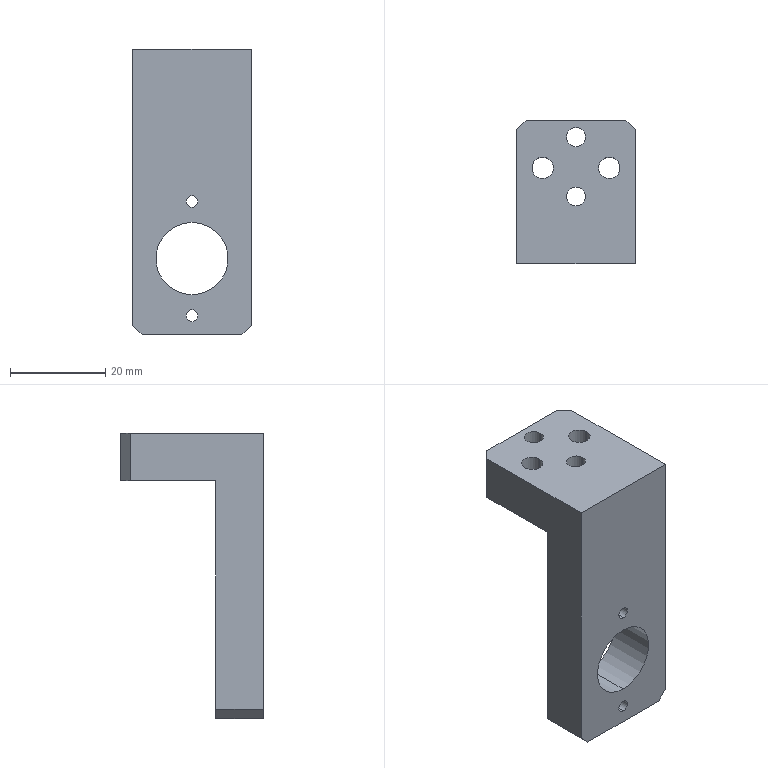Part | SolidWorks | features HoleWzd 3, ICE 2, Chamfer 1, Extrusion 1 | 1 solid | 32 faces | box 25 x 30 x 60 mm | volume 17122 mm3 | cylinder 18 | plane 14 | commonest cylinder face diameters 2.5 x4 4 x4 4.5 x4 8 x4 15.2 x2
STEP:
#1=CARTESIAN_POINT('',(0.,10.,-27.25));
#2=VERTEX_POINT('',#1);
#3=CARTESIAN_POINT('',(0.,10.,-24.75));
#4=VERTEX_POINT('',#3);
#5=CARTESIAN_POINT('',(0.,10.,-26.));
#6=DIRECTION('',(0.,1.,0.));
#7=DIRECTION('',(0.,0.,1.));
#8=AXIS2_PLACEMENT_3D('',#5,#6,#7);
#9=CIRCLE('',#8,1.25);
#10=EDGE_CURVE('',#2,#4,#9,.T.);
#11=ORIENTED_EDGE('',*,*,#10,.T.);
#12=CARTESIAN_POINT('',(0.,0.,-24.75));
#13=VERTEX_POINT('',#12);
#14=CARTESIAN_POINT('',(0.,0.,-24.75));
#15=DIRECTION('',(0.,-1.,0.));
#16=VECTOR('',#15,1000.);
#17=LINE('',#14,#16);
#18=EDGE_CURVE('',#4,#13,#17,.T.);
#19=ORIENTED_EDGE('',*,*,#18,.T.);
#20=CARTESIAN_POINT('',(0.,0.,-27.25));
#21=VERTEX_POINT('',#20);
#22=CARTESIAN_POINT('',(0.,0.,-26.));
#23=DIRECTION('',(0.,-1.,0.));
#24=DIRECTION('',(0.,0.,-1.));
#25=AXIS2_PLACEMENT_3D('',#22,#23,#24);
#26=CIRCLE('',#25,1.25);
#27=EDGE_CURVE('',#13,#21,#26,.T.);
#28=ORIENTED_EDGE('',*,*,#27,.T.);
#29=CARTESIAN_POINT('',(0.,0.,-27.25));
#30=DIRECTION('',(0.,-1.,0.));
#31=VECTOR('',#30,1000.);
#32=LINE('',#29,#31);
#33=EDGE_CURVE('',#2,#21,#32,.T.);
#34=ORIENTED_EDGE('',*,*,#33,.F.);
#35=EDGE_LOOP('',(#11,#19,#28,#34));
#36=FACE_OUTER_BOUND('',#35,.T.);
#37=CARTESIAN_POINT('',(0.,0.,-26.));
#38=DIRECTION('',(0.,-1.,0.));
#39=DIRECTION('',(0.,0.,-1.));
#40=AXIS2_PLACEMENT_3D('',#37,#38,#39);
#41=CYLINDRICAL_SURFACE('',#40,1.25);
#42=ADVANCED_FACE('',(#36),#41,.F.);
#43=CARTESIAN_POINT('',(0.,10.,-3.25));
#44=VERTEX_POINT('',#43);
#45=CARTESIAN_POINT('',(0.,10.,-0.75));
#46=VERTEX_POINT('',#45);
#47=CARTESIAN_POINT('',(0.,10.,-2.));
#48=DIRECTION('',(0.,1.,0.));
#49=DIRECTION('',(0.,0.,1.));
#50=AXIS2_PLACEMENT_3D('',#47,#48,#49);
#51=CIRCLE('',#50,1.25);
#52=EDGE_CURVE('',#44,#46,#51,.T.);
#53=ORIENTED_EDGE('',*,*,#52,.T.);
#54=CARTESIAN_POINT('',(0.,0.,-0.75));
#55=VERTEX_POINT('',#54);
#56=CARTESIAN_POINT('',(0.,0.,-0.75));
#57=DIRECTION('',(0.,-1.,0.));
#58=VECTOR('',#57,1000.);
#59=LINE('',#56,#58);
#60=EDGE_CURVE('',#46,#55,#59,.T.);
#61=ORIENTED_EDGE('',*,*,#60,.T.);
#62=CARTESIAN_POINT('',(0.,0.,-3.25));
#63=VERTEX_POINT('',#62);
#64=CARTESIAN_POINT('',(0.,0.,-2.));
#65=DIRECTION('',(0.,-1.,0.));
#66=DIRECTION('',(0.,0.,-1.));
#67=AXIS2_PLACEMENT_3D('',#64,#65,#66);
#68=CIRCLE('',#67,1.25);
#69=EDGE_CURVE('',#55,#63,#68,.T.);
#70=ORIENTED_EDGE('',*,*,#69,.T.);
#71=CARTESIAN_POINT('',(0.,0.,-3.25));
#72=DIRECTION('',(0.,-1.,0.));
#73=VECTOR('',#72,1000.);
#74=LINE('',#71,#73);
#75=EDGE_CURVE('',#44,#63,#74,.T.);
#76=ORIENTED_EDGE('',*,*,#75,.F.);
#77=EDGE_LOOP('',(#53,#61,#70,#76));
#78=FACE_OUTER_BOUND('',#77,.T.);
#79=CARTESIAN_POINT('',(0.,0.,-2.));
#80=DIRECTION('',(0.,-1.,0.));
#81=DIRECTION('',(0.,0.,-1.));
#82=AXIS2_PLACEMENT_3D('',#79,#80,#81);
#83=CYLINDRICAL_SURFACE('',#82,1.25);
#84=ADVANCED_FACE('',(#78),#83,.F.);
#85=CARTESIAN_POINT('',(2.,26.5,30.));
#86=VERTEX_POINT('',#85);
#87=CARTESIAN_POINT('',(-2.,26.5,30.));
#88=VERTEX_POINT('',#87);
#89=CARTESIAN_POINT('',(0.,26.5,30.));
#90=DIRECTION('',(0.,0.,-1.));
#91=DIRECTION('',(-1.,0.,0.));
#92=AXIS2_PLACEMENT_3D('',#89,#90,#91);
#93=CIRCLE('',#92,2.);
#94=EDGE_CURVE('',#86,#88,#93,.T.);
#95=ORIENTED_EDGE('',*,*,#94,.F.);
#96=CARTESIAN_POINT('',(2.,26.5,20.));
#97=VERTEX_POINT('',#96);
#98=CARTESIAN_POINT('',(2.,26.5,20.));
#99=DIRECTION('',(0.,0.,-1.));
#100=VECTOR('',#99,1000.);
#101=LINE('',#98,#100);
#102=EDGE_CURVE('',#86,#97,#101,.T.);
#103=ORIENTED_EDGE('',*,*,#102,.T.);
#104=CARTESIAN_POINT('',(-2.,26.5,20.));
#105=VERTEX_POINT('',#104);
#106=CARTESIAN_POINT('',(0.,26.5,20.));
#107=DIRECTION('',(0.,0.,-1.));
#108=DIRECTION('',(-1.,0.,0.));
#109=AXIS2_PLACEMENT_3D('',#106,#107,#108);
#110=CIRCLE('',#109,2.);
#111=EDGE_CURVE('',#97,#105,#110,.T.);
#112=ORIENTED_EDGE('',*,*,#111,.T.);
#113=CARTESIAN_POINT('',(-2.,26.5,20.));
#114=DIRECTION('',(0.,0.,-1.));
#115=VECTOR('',#114,1000.);
#116=LINE('',#113,#115);
#117=EDGE_CURVE('',#88,#105,#116,.T.);
#118=ORIENTED_EDGE('',*,*,#117,.F.);
#119=EDGE_LOOP('',(#95,#103,#112,#118));
#120=FACE_OUTER_BOUND('',#119,.T.);
#121=CARTESIAN_POINT('',(0.,26.5,20.));
#122=DIRECTION('',(0.,0.,-1.));
#123=DIRECTION('',(-1.,0.,0.));
#124=AXIS2_PLACEMENT_3D('',#121,#122,#123);
#125=CYLINDRICAL_SURFACE('',#124,2.);
#126=ADVANCED_FACE('',(#120),#125,.F.);
#127=CARTESIAN_POINT('',(2.,14.,30.));
#128=VERTEX_POINT('',#127);
#129=CARTESIAN_POINT('',(-2.,14.,30.));
#130=VERTEX_POINT('',#129);
#131=CARTESIAN_POINT('',(0.,14.,30.));
#132=DIRECTION('',(0.,0.,-1.));
#133=DIRECTION('',(-1.,0.,0.));
#134=AXIS2_PLACEMENT_3D('',#131,#132,#133);
#135=CIRCLE('',#134,2.);
#136=EDGE_CURVE('',#128,#130,#135,.T.);
#137=ORIENTED_EDGE('',*,*,#136,.F.);
#138=CARTESIAN_POINT('',(2.,14.,20.));
#139=VERTEX_POINT('',#138);
#140=CARTESIAN_POINT('',(2.,14.,20.));
#141=DIRECTION('',(0.,0.,-1.));
#142=VECTOR('',#141,1000.);
#143=LINE('',#140,#142);
#144=EDGE_CURVE('',#128,#139,#143,.T.);
#145=ORIENTED_EDGE('',*,*,#144,.T.);
#146=CARTESIAN_POINT('',(-2.,14.,20.));
#147=VERTEX_POINT('',#146);
#148=CARTESIAN_POINT('',(0.,14.,20.));
#149=DIRECTION('',(0.,0.,-1.));
#150=DIRECTION('',(-1.,0.,0.));
#151=AXIS2_PLACEMENT_3D('',#148,#149,#150);
#152=CIRCLE('',#151,2.);
#153=EDGE_CURVE('',#139,#147,#152,.T.);
#154=ORIENTED_EDGE('',*,*,#153,.T.);
#155=CARTESIAN_POINT('',(-2.,14.,20.));
#156=DIRECTION('',(0.,0.,-1.));
#157=VECTOR('',#156,1000.);
#158=LINE('',#155,#157);
#159=EDGE_CURVE('',#130,#147,#158,.T.);
#160=ORIENTED_EDGE('',*,*,#159,.F.);
#161=EDGE_LOOP('',(#137,#145,#154,#160));
#162=FACE_OUTER_BOUND('',#161,.T.);
#163=CARTESIAN_POINT('',(0.,14.,20.));
#164=DIRECTION('',(0.,0.,-1.));
#165=DIRECTION('',(-1.,0.,0.));
#166=AXIS2_PLACEMENT_3D('',#163,#164,#165);
#167=CYLINDRICAL_SURFACE('',#166,2.);
#168=ADVANCED_FACE('',(#162),#167,.F.);
#169=CARTESIAN_POINT('',(-3.,20.,24.6));
#170=VERTEX_POINT('',#169);
#171=CARTESIAN_POINT('',(-11.,20.,24.6));
#172=VERTEX_POINT('',#171);
#173=CARTESIAN_POINT('',(-7.,20.,24.6));
#174=DIRECTION('',(0.,0.,-1.));
#175=DIRECTION('',(-1.,0.,0.));
#176=AXIS2_PLACEMENT_3D('',#173,#174,#175);
#177=CIRCLE('',#176,4.);
#178=EDGE_CURVE('',#170,#172,#177,.T.);
#179=ORIENTED_EDGE('',*,*,#178,.F.);
#180=CARTESIAN_POINT('',(-3.,20.,20.));
#181=VERTEX_POINT('',#180);
#182=CARTESIAN_POINT('',(-3.,20.,20.));
#183=DIRECTION('',(0.,0.,-1.));
#184=VECTOR('',#183,1000.);
#185=LINE('',#182,#184);
#186=EDGE_CURVE('',#170,#181,#185,.T.);
#187=ORIENTED_EDGE('',*,*,#186,.T.);
#188=CARTESIAN_POINT('',(-11.,20.,20.));
#189=VERTEX_POINT('',#188);
#190=CARTESIAN_POINT('',(-7.,20.,20.));
#191=DIRECTION('',(0.,0.,-1.));
#192=DIRECTION('',(-1.,0.,0.));
#193=AXIS2_PLACEMENT_3D('',#190,#191,#192);
#194=CIRCLE('',#193,4.);
#195=EDGE_CURVE('',#181,#189,#194,.T.);
#196=ORIENTED_EDGE('',*,*,#195,.T.);
#197=CARTESIAN_POINT('',(-11.,20.,20.));
#198=DIRECTION('',(0.,0.,-1.));
#199=VECTOR('',#198,1000.);
#200=LINE('',#197,#199);
#201=EDGE_CURVE('',#172,#189,#200,.T.);
#202=ORIENTED_EDGE('',*,*,#201,.F.);
#203=EDGE_LOOP('',(#179,#187,#196,#202));
#204=FACE_OUTER_BOUND('',#203,.T.);
#205=CARTESIAN_POINT('',(-7.,20.,20.));
#206=DIRECTION('',(0.,0.,-1.));
#207=DIRECTION('',(-1.,0.,0.));
#208=AXIS2_PLACEMENT_3D('',#205,#206,#207);
#209=CYLINDRICAL_SURFACE('',#208,4.);
#210=ADVANCED_FACE('',(#204),#209,.F.);
#211=CARTESIAN_POINT('',(-4.75,20.,30.));
#212=VERTEX_POINT('',#211);
#213=CARTESIAN_POINT('',(-9.25,20.,30.));
#214=VERTEX_POINT('',#213);
#215=CARTESIAN_POINT('',(-7.,20.,30.));
#216=DIRECTION('',(0.,0.,-1.));
#217=DIRECTION('',(-1.,0.,0.));
#218=AXIS2_PLACEMENT_3D('',#215,#216,#217);
#219=CIRCLE('',#218,2.25);
#220=EDGE_CURVE('',#212,#214,#219,.T.);
#221=ORIENTED_EDGE('',*,*,#220,.F.);
#222=CARTESIAN_POINT('',(-4.75,20.,24.6));
#223=VERTEX_POINT('',#222);
#224=CARTESIAN_POINT('',(-4.75,20.,20.));
#225=DIRECTION('',(0.,0.,-1.));
#226=VECTOR('',#225,1000.);
#227=LINE('',#224,#226);
#228=EDGE_CURVE('',#212,#223,#227,.T.);
#229=ORIENTED_EDGE('',*,*,#228,.T.);
#230=CARTESIAN_POINT('',(-9.25,20.,24.6));
#231=VERTEX_POINT('',#230);
#232=CARTESIAN_POINT('',(-7.,20.,24.6));
#233=DIRECTION('',(0.,0.,-1.));
#234=DIRECTION('',(-1.,0.,0.));
#235=AXIS2_PLACEMENT_3D('',#232,#233,#234);
#236=CIRCLE('',#235,2.25);
#237=EDGE_CURVE('',#223,#231,#236,.T.);
#238=ORIENTED_EDGE('',*,*,#237,.T.);
#239=CARTESIAN_POINT('',(-9.25,20.,20.));
#240=DIRECTION('',(0.,0.,-1.));
#241=VECTOR('',#240,1000.);
#242=LINE('',#239,#241);
#243=EDGE_CURVE('',#214,#231,#242,.T.);
#244=ORIENTED_EDGE('',*,*,#243,.F.);
#245=EDGE_LOOP('',(#221,#229,#238,#244));
#246=FACE_OUTER_BOUND('',#245,.T.);
#247=CARTESIAN_POINT('',(-7.,20.,20.));
#248=DIRECTION('',(0.,0.,-1.));
#249=DIRECTION('',(-1.,0.,0.));
#250=AXIS2_PLACEMENT_3D('',#247,#248,#249);
#251=CYLINDRICAL_SURFACE('',#250,2.25);
#252=ADVANCED_FACE('',(#246),#251,.F.);
#253=CARTESIAN_POINT('',(11.,20.,24.6));
#254=VERTEX_POINT('',#253);
#255=CARTESIAN_POINT('',(3.,20.,24.6));
#256=VERTEX_POINT('',#255);
#257=CARTESIAN_POINT('',(7.,20.,24.6));
#258=DIRECTION('',(0.,0.,-1.));
#259=DIRECTION('',(-1.,0.,0.));
#260=AXIS2_PLACEMENT_3D('',#257,#258,#259);
#261=CIRCLE('',#260,4.);
#262=EDGE_CURVE('',#254,#256,#261,.T.);
#263=ORIENTED_EDGE('',*,*,#262,.F.);
#264=CARTESIAN_POINT('',(11.,20.,20.));
#265=VERTEX_POINT('',#264);
#266=CARTESIAN_POINT('',(11.,20.,20.));
#267=DIRECTION('',(0.,0.,-1.));
#268=VECTOR('',#267,1000.);
#269=LINE('',#266,#268);
#270=EDGE_CURVE('',#254,#265,#269,.T.);
#271=ORIENTED_EDGE('',*,*,#270,.T.);
#272=CARTESIAN_POINT('',(3.,20.,20.));
#273=VERTEX_POINT('',#272);
#274=CARTESIAN_POINT('',(7.,20.,20.));
#275=DIRECTION('',(0.,0.,-1.));
#276=DIRECTION('',(-1.,0.,0.));
#277=AXIS2_PLACEMENT_3D('',#274,#275,#276);
#278=CIRCLE('',#277,4.);
#279=EDGE_CURVE('',#265,#273,#278,.T.);
#280=ORIENTED_EDGE('',*,*,#279,.T.);
#281=CARTESIAN_POINT('',(3.,20.,20.));
#282=DIRECTION('',(0.,0.,-1.));
#283=VECTOR('',#282,1000.);
#284=LINE('',#281,#283);
#285=EDGE_CURVE('',#256,#273,#284,.T.);
#286=ORIENTED_EDGE('',*,*,#285,.F.);
#287=EDGE_LOOP('',(#263,#271,#280,#286));
#288=FACE_OUTER_BOUND('',#287,.T.);
#289=CARTESIAN_POINT('',(7.,20.,20.));
#290=DIRECTION('',(0.,0.,-1.));
#291=DIRECTION('',(-1.,0.,0.));
#292=AXIS2_PLACEMENT_3D('',#289,#290,#291);
#293=CYLINDRICAL_SURFACE('',#292,4.);
#294=ADVANCED_FACE('',(#288),#293,.F.);
#295=CARTESIAN_POINT('',(9.25,20.,30.));
#296=VERTEX_POINT('',#295);
#297=CARTESIAN_POINT('',(4.75,20.,30.));
#298=VERTEX_POINT('',#297);
#299=CARTESIAN_POINT('',(7.,20.,30.));
#300=DIRECTION('',(0.,0.,-1.));
#301=DIRECTION('',(-1.,0.,0.));
#302=AXIS2_PLACEMENT_3D('',#299,#300,#301);
#303=CIRCLE('',#302,2.25);
#304=EDGE_CURVE('',#296,#298,#303,.T.);
#305=ORIENTED_EDGE('',*,*,#304,.F.);
#306=CARTESIAN_POINT('',(9.25,20.,24.6));
#307=VERTEX_POINT('',#306);
#308=CARTESIAN_POINT('',(9.25,20.,20.));
#309=DIRECTION('',(0.,0.,-1.));
#310=VECTOR('',#309,1000.);
#311=LINE('',#308,#310);
#312=EDGE_CURVE('',#296,#307,#311,.T.);
#313=ORIENTED_EDGE('',*,*,#312,.T.);
#314=CARTESIAN_POINT('',(4.75,20.,24.6));
#315=VERTEX_POINT('',#314);
#316=CARTESIAN_POINT('',(7.,20.,24.6));
#317=DIRECTION('',(0.,0.,-1.));
#318=DIRECTION('',(-1.,0.,0.));
#319=AXIS2_PLACEMENT_3D('',#316,#317,#318);
#320=CIRCLE('',#319,2.25);
#321=EDGE_CURVE('',#307,#315,#320,.T.);
#322=ORIENTED_EDGE('',*,*,#321,.T.);
#323=CARTESIAN_POINT('',(4.75,20.,20.));
#324=DIRECTION('',(0.,0.,-1.));
#325=VECTOR('',#324,1000.);
#326=LINE('',#323,#325);
#327=EDGE_CURVE('',#298,#315,#326,.T.);
#328=ORIENTED_EDGE('',*,*,#327,.F.);
#329=EDGE_LOOP('',(#305,#313,#322,#328));
#330=FACE_OUTER_BOUND('',#329,.T.);
#331=CARTESIAN_POINT('',(7.,20.,20.));
#332=DIRECTION('',(0.,0.,-1.));
#333=DIRECTION('',(-1.,0.,0.));
#334=AXIS2_PLACEMENT_3D('',#331,#332,#333);
#335=CYLINDRICAL_SURFACE('',#334,2.25);
#336=ADVANCED_FACE('',(#330),#335,.F.);
#337=CARTESIAN_POINT('',(0.,10.,-21.6));
#338=VERTEX_POINT('',#337);
#339=CARTESIAN_POINT('',(0.,10.,-6.4));
#340=VERTEX_POINT('',#339);
#341=CARTESIAN_POINT('',(0.,10.,-14.));
#342=DIRECTION('',(0.,1.,0.));
#343=DIRECTION('',(0.,0.,1.));
#344=AXIS2_PLACEMENT_3D('',#341,#342,#343);
#345=CIRCLE('',#344,7.6);
#346=EDGE_CURVE('',#338,#340,#345,.T.);
#347=ORIENTED_EDGE('',*,*,#346,.T.);
#348=CARTESIAN_POINT('',(0.,0.,-6.4));
#349=VERTEX_POINT('',#348);
#350=CARTESIAN_POINT('',(0.,20.,-6.4));
#351=DIRECTION('',(0.,-1.,0.));
#352=VECTOR('',#351,1000.);
#353=LINE('',#350,#352);
#354=EDGE_CURVE('',#340,#349,#353,.T.);
#355=ORIENTED_EDGE('',*,*,#354,.T.);
#356=CARTESIAN_POINT('',(0.,0.,-21.6));
#357=VERTEX_POINT('',#356);
#358=CARTESIAN_POINT('',(0.,0.,-14.));
#359=DIRECTION('',(0.,-1.,0.));
#360=DIRECTION('',(0.,0.,-1.));
#361=AXIS2_PLACEMENT_3D('',#358,#359,#360);
#362=CIRCLE('',#361,7.6);
#363=EDGE_CURVE('',#349,#357,#362,.T.);
#364=ORIENTED_EDGE('',*,*,#363,.T.);
#365=CARTESIAN_POINT('',(0.,20.,-21.6));
#366=DIRECTION('',(0.,-1.,0.));
#367=VECTOR('',#366,1000.);
#368=LINE('',#365,#367);
#369=EDGE_CURVE('',#338,#357,#368,.T.);
#370=ORIENTED_EDGE('',*,*,#369,.F.);
#371=EDGE_LOOP('',(#347,#355,#364,#370));
#372=FACE_OUTER_BOUND('',#371,.T.);
#373=CARTESIAN_POINT('',(0.,20.,-14.));
#374=DIRECTION('',(0.,-1.,0.));
#375=DIRECTION('',(0.,0.,-1.));
#376=AXIS2_PLACEMENT_3D('',#373,#374,#375);
#377=CYLINDRICAL_SURFACE('',#376,7.6);
#378=ADVANCED_FACE('',(#372),#377,.F.);
#379=CARTESIAN_POINT('',(12.5,28.,20.));
#380=VERTEX_POINT('',#379);
#381=CARTESIAN_POINT('',(12.5,10.,20.));
#382=VERTEX_POINT('',#381);
#383=CARTESIAN_POINT('',(12.5,30.,20.));
#384=DIRECTION('',(0.,-1.,0.));
#385=VECTOR('',#384,1000.);
#386=LINE('',#383,#385);
#387=EDGE_CURVE('',#380,#382,#386,.T.);
#388=ORIENTED_EDGE('',*,*,#387,.F.);
#389=CARTESIAN_POINT('',(12.5,28.,30.));
#390=VERTEX_POINT('',#389);
#391=CARTESIAN_POINT('',(12.5,28.,-30.));
#392=DIRECTION('',(0.,0.,1.));
#393=VECTOR('',#392,1000.);
#394=LINE('',#391,#393);
#395=EDGE_CURVE('',#380,#390,#394,.T.);
#396=ORIENTED_EDGE('',*,*,#395,.T.);
#397=CARTESIAN_POINT('',(12.5,0.,30.));
#398=VERTEX_POINT('',#397);
#399=CARTESIAN_POINT('',(12.5,10.,30.));
#400=DIRECTION('',(0.,-1.,0.));
#401=VECTOR('',#400,1000.);
#402=LINE('',#399,#401);
#403=EDGE_CURVE('',#390,#398,#402,.T.);
#404=ORIENTED_EDGE('',*,*,#403,.T.);
#405=CARTESIAN_POINT('',(12.5,0.,-28.));
#406=VERTEX_POINT('',#405);
#407=CARTESIAN_POINT('',(12.5,0.,-30.));
#408=DIRECTION('',(0.,0.,-1.));
#409=VECTOR('',#408,1000.);
#410=LINE('',#407,#409);
#411=EDGE_CURVE('',#398,#406,#410,.T.);
#412=ORIENTED_EDGE('',*,*,#411,.T.);
#413=CARTESIAN_POINT('',(12.5,10.,-28.));
#414=VERTEX_POINT('',#413);
#415=CARTESIAN_POINT('',(12.5,10.,-28.));
#416=DIRECTION('',(0.,1.,0.));
#417=VECTOR('',#416,1000.);
#418=LINE('',#415,#417);
#419=EDGE_CURVE('',#406,#414,#418,.T.);
#420=ORIENTED_EDGE('',*,*,#419,.T.);
#421=CARTESIAN_POINT('',(12.5,10.,-30.));
#422=DIRECTION('',(0.,0.,-1.));
#423=VECTOR('',#422,1000.);
#424=LINE('',#421,#423);
#425=EDGE_CURVE('',#382,#414,#424,.T.);
#426=ORIENTED_EDGE('',*,*,#425,.F.);
#427=EDGE_LOOP('',(#388,#396,#404,#412,#420,#426));
#428=FACE_OUTER_BOUND('',#427,.T.);
#429=CARTESIAN_POINT('',(12.5,10.,-30.));
#430=DIRECTION('',(-1.,0.,0.));
#431=DIRECTION('',(0.,0.,1.));
#432=AXIS2_PLACEMENT_3D('',#429,#430,#431);
#433=PLANE('',#432);
#434=ADVANCED_FACE('',(#428),#433,.F.);
#435=CARTESIAN_POINT('',(10.5,0.,-30.));
#436=VERTEX_POINT('',#435);
#437=CARTESIAN_POINT('',(-10.5,0.,-30.));
#438=VERTEX_POINT('',#437);
#439=CARTESIAN_POINT('',(-12.5,0.,-30.));
#440=DIRECTION('',(-1.,0.,0.));
#441=VECTOR('',#440,1000.);
#442=LINE('',#439,#441);
#443=EDGE_CURVE('',#436,#438,#442,.T.);
#444=ORIENTED_EDGE('',*,*,#443,.T.);
#445=CARTESIAN_POINT('',(-10.5,10.,-30.));
#446=VERTEX_POINT('',#445);
#447=CARTESIAN_POINT('',(-10.5,10.,-30.));
#448=DIRECTION('',(0.,1.,0.));
#449=VECTOR('',#448,1000.);
#450=LINE('',#447,#449);
#451=EDGE_CURVE('',#438,#446,#450,.T.);
#452=ORIENTED_EDGE('',*,*,#451,.T.);
#453=CARTESIAN_POINT('',(10.5,10.,-30.));
#454=VERTEX_POINT('',#453);
#455=CARTESIAN_POINT('',(-12.5,10.,-30.));
#456=DIRECTION('',(-1.,0.,0.));
#457=VECTOR('',#456,1000.);
#458=LINE('',#455,#457);
#459=EDGE_CURVE('',#454,#446,#458,.T.);
#460=ORIENTED_EDGE('',*,*,#459,.F.);
#461=CARTESIAN_POINT('',(10.5,10.,-30.));
#462=DIRECTION('',(0.,-1.,0.));
#463=VECTOR('',#462,1000.);
#464=LINE('',#461,#463);
#465=EDGE_CURVE('',#454,#436,#464,.T.);
#466=ORIENTED_EDGE('',*,*,#465,.T.);
#467=EDGE_LOOP('',(#444,#452,#460,#466));
#468=FACE_OUTER_BOUND('',#467,.T.);
#469=CARTESIAN_POINT('',(-12.5,10.,-30.));
#470=DIRECTION('',(0.,0.,1.));
#471=DIRECTION('',(1.,0.,0.));
#472=AXIS2_PLACEMENT_3D('',#469,#470,#471);
#473=PLANE('',#472);
#474=ADVANCED_FACE('',(#468),#473,.F.);
#475=CARTESIAN_POINT('',(-12.5,28.,30.));
#476=VERTEX_POINT('',#475);
#477=CARTESIAN_POINT('',(-12.5,0.,30.));
#478=VERTEX_POINT('',#477);
#479=CARTESIAN_POINT('',(-12.5,10.,30.));
#480=DIRECTION('',(0.,-1.,0.));
#481=VECTOR('',#480,1000.);
#482=LINE('',#479,#481);
#483=EDGE_CURVE('',#476,#478,#482,.T.);
#484=ORIENTED_EDGE('',*,*,#483,.F.);
#485=CARTESIAN_POINT('',(-12.5,28.,20.));
#486=VERTEX_POINT('',#485);
#487=CARTESIAN_POINT('',(-12.5,28.,-30.));
#488=DIRECTION('',(0.,0.,-1.));
#489=VECTOR('',#488,1000.);
#490=LINE('',#487,#489);
#491=EDGE_CURVE('',#476,#486,#490,.T.);
#492=ORIENTED_EDGE('',*,*,#491,.T.);
#493=CARTESIAN_POINT('',(-12.5,10.,20.));
#494=VERTEX_POINT('',#493);
#495=CARTESIAN_POINT('',(-12.5,30.,20.));
#496=DIRECTION('',(0.,-1.,0.));
#497=VECTOR('',#496,1000.);
#498=LINE('',#495,#497);
#499=EDGE_CURVE('',#486,#494,#498,.T.);
#500=ORIENTED_EDGE('',*,*,#499,.T.);
#501=CARTESIAN_POINT('',(-12.5,10.,-28.));
#502=VERTEX_POINT('',#501);
#503=CARTESIAN_POINT('',(-12.5,10.,-30.));
#504=DIRECTION('',(0.,0.,1.));
#505=VECTOR('',#504,1000.);
#506=LINE('',#503,#505);
#507=EDGE_CURVE('',#502,#494,#506,.T.);
#508=ORIENTED_EDGE('',*,*,#507,.F.);
#509=CARTESIAN_POINT('',(-12.5,0.,-28.));
#510=VERTEX_POINT('',#509);
#511=CARTESIAN_POINT('',(-12.5,10.,-28.));
#512=DIRECTION('',(0.,-1.,0.));
#513=VECTOR('',#512,1000.);
#514=LINE('',#511,#513);
#515=EDGE_CURVE('',#502,#510,#514,.T.);
#516=ORIENTED_EDGE('',*,*,#515,.T.);
#517=CARTESIAN_POINT('',(-12.5,0.,-30.));
#518=DIRECTION('',(0.,0.,1.));
#519=VECTOR('',#518,1000.);
#520=LINE('',#517,#519);
#521=EDGE_CURVE('',#510,#478,#520,.T.);
#522=ORIENTED_EDGE('',*,*,#521,.T.);
#523=EDGE_LOOP('',(#484,#492,#500,#508,#516,#522));
#524=FACE_OUTER_BOUND('',#523,.T.);
#525=CARTESIAN_POINT('',(-12.5,10.,-30.));
#526=DIRECTION('',(1.,0.,0.));
#527=DIRECTION('',(0.,0.,-1.));
#528=AXIS2_PLACEMENT_3D('',#525,#526,#527);
#529=PLANE('',#528);
#530=ADVANCED_FACE('',(#524),#529,.F.);
#531=CARTESIAN_POINT('',(0.,26.5,30.));
#532=DIRECTION('',(0.,0.,-1.));
#533=DIRECTION('',(-1.,0.,0.));
#534=AXIS2_PLACEMENT_3D('',#531,#532,#533);
#535=CIRCLE('',#534,2.);
#536=EDGE_CURVE('',#88,#86,#535,.T.);
#537=ORIENTED_EDGE('',*,*,#536,.T.);
#538=ORIENTED_EDGE('',*,*,#94,.T.);
#539=EDGE_LOOP('',(#537,#538));
#540=FACE_BOUND('',#539,.T.);
#541=CARTESIAN_POINT('',(0.,14.,30.));
#542=DIRECTION('',(0.,0.,-1.));
#543=DIRECTION('',(-1.,0.,0.));
#544=AXIS2_PLACEMENT_3D('',#541,#542,#543);
#545=CIRCLE('',#544,2.);
#546=EDGE_CURVE('',#130,#128,#545,.T.);
#547=ORIENTED_EDGE('',*,*,#546,.T.);
#548=ORIENTED_EDGE('',*,*,#136,.T.);
#549=EDGE_LOOP('',(#547,#548));
#550=FACE_BOUND('',#549,.T.);
#551=CARTESIAN_POINT('',(-7.,20.,30.));
#552=DIRECTION('',(0.,0.,-1.));
#553=DIRECTION('',(-1.,0.,0.));
#554=AXIS2_PLACEMENT_3D('',#551,#552,#553);
#555=CIRCLE('',#554,2.25);
#556=EDGE_CURVE('',#214,#212,#555,.T.);
#557=ORIENTED_EDGE('',*,*,#556,.T.);
#558=ORIENTED_EDGE('',*,*,#220,.T.);
#559=EDGE_LOOP('',(#557,#558));
#560=FACE_BOUND('',#559,.T.);
#561=CARTESIAN_POINT('',(7.,20.,30.));
#562=DIRECTION('',(0.,0.,-1.));
#563=DIRECTION('',(-1.,0.,0.));
#564=AXIS2_PLACEMENT_3D('',#561,#562,#563);
#565=CIRCLE('',#564,2.25);
#566=EDGE_CURVE('',#298,#296,#565,.T.);
#567=ORIENTED_EDGE('',*,*,#566,.T.);
#568=ORIENTED_EDGE('',*,*,#304,.T.);
#569=EDGE_LOOP('',(#567,#568));
#570=FACE_BOUND('',#569,.T.);
#571=CARTESIAN_POINT('',(-10.5,30.,30.));
#572=VERTEX_POINT('',#571);
#573=CARTESIAN_POINT('',(10.5,30.,30.));
#574=VERTEX_POINT('',#573);
#575=CARTESIAN_POINT('',(-12.5,30.,30.));
#576=DIRECTION('',(1.,0.,0.));
#577=VECTOR('',#576,1000.);
#578=LINE('',#575,#577);
#579=EDGE_CURVE('',#572,#574,#578,.T.);
#580=ORIENTED_EDGE('',*,*,#579,.F.);
#581=CARTESIAN_POINT('',(-10.5,30.,30.));
#582=DIRECTION('',(-0.7071,-0.7071,0.));
#583=VECTOR('',#582,1000.);
#584=LINE('',#581,#583);
#585=EDGE_CURVE('',#572,#476,#584,.T.);
#586=ORIENTED_EDGE('',*,*,#585,.T.);
#587=ORIENTED_EDGE('',*,*,#483,.T.);
#588=CARTESIAN_POINT('',(-12.5,0.,30.));
#589=DIRECTION('',(1.,0.,0.));
#590=VECTOR('',#589,1000.);
#591=LINE('',#588,#590);
#592=EDGE_CURVE('',#478,#398,#591,.T.);
#593=ORIENTED_EDGE('',*,*,#592,.T.);
#594=ORIENTED_EDGE('',*,*,#403,.F.);
#595=CARTESIAN_POINT('',(10.5,30.,30.));
#596=DIRECTION('',(-0.7071,0.7071,0.));
#597=VECTOR('',#596,1000.);
#598=LINE('',#595,#597);
#599=EDGE_CURVE('',#390,#574,#598,.T.);
#600=ORIENTED_EDGE('',*,*,#599,.T.);
#601=EDGE_LOOP('',(#580,#586,#587,#593,#594,#600));
#602=FACE_OUTER_BOUND('',#601,.T.);
#603=CARTESIAN_POINT('',(-12.5,10.,30.));
#604=DIRECTION('',(0.,0.,-1.));
#605=DIRECTION('',(-1.,0.,0.));
#606=AXIS2_PLACEMENT_3D('',#603,#604,#605);
#607=PLANE('',#606);
#608=ADVANCED_FACE('',(#540,#550,#560,#570,#602),#607,.F.);
#609=ORIENTED_EDGE('',*,*,#10,.F.);
#610=CARTESIAN_POINT('',(0.,10.,-26.));
#611=DIRECTION('',(0.,1.,0.));
#612=DIRECTION('',(0.,0.,1.));
#613=AXIS2_PLACEMENT_3D('',#610,#611,#612);
#614=CIRCLE('',#613,1.25);
#615=EDGE_CURVE('',#4,#2,#614,.T.);
#616=ORIENTED_EDGE('',*,*,#615,.F.);
#617=EDGE_LOOP('',(#609,#616));
#618=FACE_BOUND('',#617,.T.);
#619=ORIENTED_EDGE('',*,*,#52,.F.);
#620=CARTESIAN_POINT('',(0.,10.,-2.));
#621=DIRECTION('',(0.,1.,0.));
#622=DIRECTION('',(0.,0.,1.));
#623=AXIS2_PLACEMENT_3D('',#620,#621,#622);
#624=CIRCLE('',#623,1.25);
#625=EDGE_CURVE('',#46,#44,#624,.T.);
#626=ORIENTED_EDGE('',*,*,#625,.F.);
#627=EDGE_LOOP('',(#619,#626));
#628=FACE_BOUND('',#627,.T.);
#629=ORIENTED_EDGE('',*,*,#459,.T.);
#630=CARTESIAN_POINT('',(-20.25,10.,-20.25));
#631=DIRECTION('',(-0.7071,0.,0.7071));
#632=VECTOR('',#631,1000.);
#633=LINE('',#630,#632);
#634=EDGE_CURVE('',#446,#502,#633,.T.);
#635=ORIENTED_EDGE('',*,*,#634,.T.);
#636=ORIENTED_EDGE('',*,*,#507,.T.);
#637=CARTESIAN_POINT('',(-12.5,10.,20.));
#638=DIRECTION('',(-1.,0.,0.));
#639=VECTOR('',#638,1000.);
#640=LINE('',#637,#639);
#641=EDGE_CURVE('',#382,#494,#640,.T.);
#642=ORIENTED_EDGE('',*,*,#641,.F.);
#643=ORIENTED_EDGE('',*,*,#425,.T.);
#644=CARTESIAN_POINT('',(20.25,10.,-20.25));
#645=DIRECTION('',(-0.7071,0.,-0.7071));
#646=VECTOR('',#645,1000.);
#647=LINE('',#644,#646);
#648=EDGE_CURVE('',#414,#454,#647,.T.);
#649=ORIENTED_EDGE('',*,*,#648,.T.);
#650=EDGE_LOOP('',(#629,#635,#636,#642,#643,#649));
#651=FACE_OUTER_BOUND('',#650,.T.);
#652=ORIENTED_EDGE('',*,*,#346,.F.);
#653=CARTESIAN_POINT('',(0.,10.,-14.));
#654=DIRECTION('',(0.,1.,0.));
#655=DIRECTION('',(0.,0.,1.));
#656=AXIS2_PLACEMENT_3D('',#653,#654,#655);
#657=CIRCLE('',#656,7.6);
#658=EDGE_CURVE('',#340,#338,#657,.T.);
#659=ORIENTED_EDGE('',*,*,#658,.F.);
#660=EDGE_LOOP('',(#652,#659));
#661=FACE_BOUND('',#660,.T.);
#662=CARTESIAN_POINT('',(0.,10.,0.));
#663=DIRECTION('',(0.,1.,0.));
#664=DIRECTION('',(0.,0.,1.));
#665=AXIS2_PLACEMENT_3D('',#662,#663,#664);
#666=PLANE('',#665);
#667=ADVANCED_FACE('',(#618,#628,#651,#661),#666,.T.);
#668=CARTESIAN_POINT('',(0.,0.,-26.));
#669=DIRECTION('',(0.,-1.,0.));
#670=DIRECTION('',(0.,0.,-1.));
#671=AXIS2_PLACEMENT_3D('',#668,#669,#670);
#672=CIRCLE('',#671,1.25);
#673=EDGE_CURVE('',#21,#13,#672,.T.);
#674=ORIENTED_EDGE('',*,*,#673,.F.);
#675=ORIENTED_EDGE('',*,*,#27,.F.);
#676=EDGE_LOOP('',(#674,#675));
#677=FACE_BOUND('',#676,.T.);
#678=CARTESIAN_POINT('',(0.,0.,-2.));
#679=DIRECTION('',(0.,-1.,0.));
#680=DIRECTION('',(0.,0.,-1.));
#681=AXIS2_PLACEMENT_3D('',#678,#679,#680);
#682=CIRCLE('',#681,1.25);
#683=EDGE_CURVE('',#63,#55,#682,.T.);
#684=ORIENTED_EDGE('',*,*,#683,.F.);
#685=ORIENTED_EDGE('',*,*,#69,.F.);
#686=EDGE_LOOP('',(#684,#685));
#687=FACE_BOUND('',#686,.T.);
#688=CARTESIAN_POINT('',(0.,0.,-14.));
#689=DIRECTION('',(0.,-1.,0.));
#690=DIRECTION('',(0.,0.,-1.));
#691=AXIS2_PLACEMENT_3D('',#688,#689,#690);
#692=CIRCLE('',#691,7.6);
#693=EDGE_CURVE('',#357,#349,#692,.T.);
#694=ORIENTED_EDGE('',*,*,#693,.F.);
#695=ORIENTED_EDGE('',*,*,#363,.F.);
#696=EDGE_LOOP('',(#694,#695));
#697=FACE_BOUND('',#696,.T.);
#698=ORIENTED_EDGE('',*,*,#521,.F.);
#699=CARTESIAN_POINT('',(-12.5,0.,-28.));
#700=DIRECTION('',(0.7071,0.,-0.7071));
#701=VECTOR('',#700,1000.);
#702=LINE('',#699,#701);
#703=EDGE_CURVE('',#510,#438,#702,.T.);
#704=ORIENTED_EDGE('',*,*,#703,.T.);
#705=ORIENTED_EDGE('',*,*,#443,.F.);
#706=CARTESIAN_POINT('',(10.5,0.,-30.));
#707=DIRECTION('',(0.7071,0.,0.7071));
#708=VECTOR('',#707,1000.);
#709=LINE('',#706,#708);
#710=EDGE_CURVE('',#436,#406,#709,.T.);
#711=ORIENTED_EDGE('',*,*,#710,.T.);
#712=ORIENTED_EDGE('',*,*,#411,.F.);
#713=ORIENTED_EDGE('',*,*,#592,.F.);
#714=EDGE_LOOP('',(#698,#704,#705,#711,#712,#713));
#715=FACE_OUTER_BOUND('',#714,.T.);
#716=CARTESIAN_POINT('',(0.,0.,0.));
#717=DIRECTION('',(0.,1.,0.));
#718=DIRECTION('',(0.,0.,1.));
#719=AXIS2_PLACEMENT_3D('',#716,#717,#718);
#720=PLANE('',#719);
#721=ADVANCED_FACE('',(#677,#687,#697,#715),#720,.F.);
#722=ORIENTED_EDGE('',*,*,#354,.F.);
#723=ORIENTED_EDGE('',*,*,#658,.T.);
#724=ORIENTED_EDGE('',*,*,#369,.T.);
#725=ORIENTED_EDGE('',*,*,#693,.T.);
#726=EDGE_LOOP('',(#722,#723,#724,#725));
#727=FACE_OUTER_BOUND('',#726,.T.);
#728=CARTESIAN_POINT('',(0.,20.,-14.));
#729=DIRECTION('',(0.,-1.,0.));
#730=DIRECTION('',(0.,0.,-1.));
#731=AXIS2_PLACEMENT_3D('',#728,#729,#730);
#732=CYLINDRICAL_SURFACE('',#731,7.6);
#733=ADVANCED_FACE('',(#727),#732,.F.);
#734=CARTESIAN_POINT('',(0.,26.5,20.));
#735=DIRECTION('',(0.,0.,-1.));
#736=DIRECTION('',(-1.,0.,0.));
#737=AXIS2_PLACEMENT_3D('',#734,#735,#736);
#738=CIRCLE('',#737,2.);
#739=EDGE_CURVE('',#105,#97,#738,.T.);
#740=ORIENTED_EDGE('',*,*,#739,.F.);
#741=ORIENTED_EDGE('',*,*,#111,.F.);
#742=EDGE_LOOP('',(#740,#741));
#743=FACE_BOUND('',#742,.T.);
#744=CARTESIAN_POINT('',(0.,14.,20.));
#745=DIRECTION('',(0.,0.,-1.));
#746=DIRECTION('',(-1.,0.,0.));
#747=AXIS2_PLACEMENT_3D('',#744,#745,#746);
#748=CIRCLE('',#747,2.);
#749=EDGE_CURVE('',#147,#139,#748,.T.);
#750=ORIENTED_EDGE('',*,*,#749,.F.);
#751=ORIENTED_EDGE('',*,*,#153,.F.);
#752=EDGE_LOOP('',(#750,#751));
#753=FACE_BOUND('',#752,.T.);
#754=CARTESIAN_POINT('',(-7.,20.,20.));
#755=DIRECTION('',(0.,0.,-1.));
#756=DIRECTION('',(-1.,0.,0.));
#757=AXIS2_PLACEMENT_3D('',#754,#755,#756);
#758=CIRCLE('',#757,4.);
#759=EDGE_CURVE('',#189,#181,#758,.T.);
#760=ORIENTED_EDGE('',*,*,#759,.F.);
#761=ORIENTED_EDGE('',*,*,#195,.F.);
#762=EDGE_LOOP('',(#760,#761));
#763=FACE_BOUND('',#762,.T.);
#764=CARTESIAN_POINT('',(7.,20.,20.));
#765=DIRECTION('',(0.,0.,-1.));
#766=DIRECTION('',(-1.,0.,0.));
#767=AXIS2_PLACEMENT_3D('',#764,#765,#766);
#768=CIRCLE('',#767,4.);
#769=EDGE_CURVE('',#273,#265,#768,.T.);
#770=ORIENTED_EDGE('',*,*,#769,.F.);
#771=ORIENTED_EDGE('',*,*,#279,.F.);
#772=EDGE_LOOP('',(#770,#771));
#773=FACE_BOUND('',#772,.T.);
#774=ORIENTED_EDGE('',*,*,#499,.F.);
#775=CARTESIAN_POINT('',(-10.5,30.,20.));
#776=VERTEX_POINT('',#775);
#777=CARTESIAN_POINT('',(-10.5,30.,20.));
#778=DIRECTION('',(0.7071,0.7071,0.));
#779=VECTOR('',#778,1000.);
#780=LINE('',#777,#779);
#781=EDGE_CURVE('',#486,#776,#780,.T.);
#782=ORIENTED_EDGE('',*,*,#781,.T.);
#783=CARTESIAN_POINT('',(10.5,30.,20.));
#784=VERTEX_POINT('',#783);
#785=CARTESIAN_POINT('',(-12.5,30.,20.));
#786=DIRECTION('',(-1.,0.,0.));
#787=VECTOR('',#786,1000.);
#788=LINE('',#785,#787);
#789=EDGE_CURVE('',#784,#776,#788,.T.);
#790=ORIENTED_EDGE('',*,*,#789,.F.);
#791=CARTESIAN_POINT('',(10.5,30.,20.));
#792=DIRECTION('',(0.7071,-0.7071,0.));
#793=VECTOR('',#792,1000.);
#794=LINE('',#791,#793);
#795=EDGE_CURVE('',#784,#380,#794,.T.);
#796=ORIENTED_EDGE('',*,*,#795,.T.);
#797=ORIENTED_EDGE('',*,*,#387,.T.);
#798=ORIENTED_EDGE('',*,*,#641,.T.);
#799=EDGE_LOOP('',(#774,#782,#790,#796,#797,#798));
#800=FACE_OUTER_BOUND('',#799,.T.);
#801=CARTESIAN_POINT('',(-12.5,30.,20.));
#802=DIRECTION('',(0.,0.,1.));
#803=DIRECTION('',(1.,0.,0.));
#804=AXIS2_PLACEMENT_3D('',#801,#802,#803);
#805=PLANE('',#804);
#806=ADVANCED_FACE('',(#743,#753,#763,#773,#800),#805,.F.);
#807=ORIENTED_EDGE('',*,*,#789,.T.);
#808=CARTESIAN_POINT('',(-10.5,30.,0.));
#809=DIRECTION('',(0.,0.,1.));
#810=VECTOR('',#809,1000.);
#811=LINE('',#808,#810);
#812=EDGE_CURVE('',#776,#572,#811,.T.);
#813=ORIENTED_EDGE('',*,*,#812,.T.);
#814=ORIENTED_EDGE('',*,*,#579,.T.);
#815=CARTESIAN_POINT('',(10.5,30.,0.));
#816=DIRECTION('',(0.,0.,-1.));
#817=VECTOR('',#816,1000.);
#818=LINE('',#815,#817);
#819=EDGE_CURVE('',#574,#784,#818,.T.);
#820=ORIENTED_EDGE('',*,*,#819,.T.);
#821=EDGE_LOOP('',(#807,#813,#814,#820));
#822=FACE_OUTER_BOUND('',#821,.T.);
#823=CARTESIAN_POINT('',(0.,30.,0.));
#824=DIRECTION('',(0.,-1.,0.));
#825=DIRECTION('',(0.,0.,-1.));
#826=AXIS2_PLACEMENT_3D('',#823,#824,#825);
#827=PLANE('',#826);
#828=ADVANCED_FACE('',(#822),#827,.F.);
#829=ORIENTED_EDGE('',*,*,#781,.F.);
#830=ORIENTED_EDGE('',*,*,#491,.F.);
#831=ORIENTED_EDGE('',*,*,#585,.F.);
#832=ORIENTED_EDGE('',*,*,#812,.F.);
#833=EDGE_LOOP('',(#829,#830,#831,#832));
#834=FACE_OUTER_BOUND('',#833,.T.);
#835=CARTESIAN_POINT('',(-10.5,30.,0.));
#836=DIRECTION('',(0.7071,-0.7071,0.));
#837=DIRECTION('',(0.,0.,1.));
#838=AXIS2_PLACEMENT_3D('',#835,#836,#837);
#839=PLANE('',#838);
#840=ADVANCED_FACE('',(#834),#839,.F.);
#841=ORIENTED_EDGE('',*,*,#599,.F.);
#842=ORIENTED_EDGE('',*,*,#395,.F.);
#843=ORIENTED_EDGE('',*,*,#795,.F.);
#844=ORIENTED_EDGE('',*,*,#819,.F.);
#845=EDGE_LOOP('',(#841,#842,#843,#844));
#846=FACE_OUTER_BOUND('',#845,.T.);
#847=CARTESIAN_POINT('',(10.5,30.,0.));
#848=DIRECTION('',(-0.7071,-0.7071,0.));
#849=DIRECTION('',(0.,0.,-1.));
#850=AXIS2_PLACEMENT_3D('',#847,#848,#849);
#851=PLANE('',#850);
#852=ADVANCED_FACE('',(#846),#851,.F.);
#853=ORIENTED_EDGE('',*,*,#634,.F.);
#854=ORIENTED_EDGE('',*,*,#451,.F.);
#855=ORIENTED_EDGE('',*,*,#703,.F.);
#856=ORIENTED_EDGE('',*,*,#515,.F.);
#857=EDGE_LOOP('',(#853,#854,#855,#856));
#858=FACE_OUTER_BOUND('',#857,.T.);
#859=CARTESIAN_POINT('',(-12.5,10.,-28.));
#860=DIRECTION('',(0.7071,0.,0.7071));
#861=DIRECTION('',(0.,-1.,0.));
#862=AXIS2_PLACEMENT_3D('',#859,#860,#861);
#863=PLANE('',#862);
#864=ADVANCED_FACE('',(#858),#863,.F.);
#865=ORIENTED_EDGE('',*,*,#648,.F.);
#866=ORIENTED_EDGE('',*,*,#419,.F.);
#867=ORIENTED_EDGE('',*,*,#710,.F.);
#868=ORIENTED_EDGE('',*,*,#465,.F.);
#869=EDGE_LOOP('',(#865,#866,#867,#868));
#870=FACE_OUTER_BOUND('',#869,.T.);
#871=CARTESIAN_POINT('',(10.5,10.,-30.));
#872=DIRECTION('',(-0.7071,0.,0.7071));
#873=DIRECTION('',(0.,-1.,0.));
#874=AXIS2_PLACEMENT_3D('',#871,#872,#873);
#875=PLANE('',#874);
#876=ADVANCED_FACE('',(#870),#875,.F.);
#877=ORIENTED_EDGE('',*,*,#312,.F.);
#878=ORIENTED_EDGE('',*,*,#566,.F.);
#879=ORIENTED_EDGE('',*,*,#327,.T.);
#880=CARTESIAN_POINT('',(7.,20.,24.6));
#881=DIRECTION('',(0.,0.,-1.));
#882=DIRECTION('',(-1.,0.,0.));
#883=AXIS2_PLACEMENT_3D('',#880,#881,#882);
#884=CIRCLE('',#883,2.25);
#885=EDGE_CURVE('',#315,#307,#884,.T.);
#886=ORIENTED_EDGE('',*,*,#885,.T.);
#887=EDGE_LOOP('',(#877,#878,#879,#886));
#888=FACE_OUTER_BOUND('',#887,.T.);
#889=CARTESIAN_POINT('',(7.,20.,20.));
#890=DIRECTION('',(0.,0.,-1.));
#891=DIRECTION('',(-1.,0.,0.));
#892=AXIS2_PLACEMENT_3D('',#889,#890,#891);
#893=CYLINDRICAL_SURFACE('',#892,2.25);
#894=ADVANCED_FACE('',(#888),#893,.F.);
#895=ORIENTED_EDGE('',*,*,#885,.F.);
#896=ORIENTED_EDGE('',*,*,#321,.F.);
#897=EDGE_LOOP('',(#895,#896));
#898=FACE_BOUND('',#897,.T.);
#899=CARTESIAN_POINT('',(7.,20.,24.6));
#900=DIRECTION('',(0.,0.,-1.));
#901=DIRECTION('',(-1.,0.,0.));
#902=AXIS2_PLACEMENT_3D('',#899,#900,#901);
#903=CIRCLE('',#902,4.);
#904=EDGE_CURVE('',#256,#254,#903,.T.);
#905=ORIENTED_EDGE('',*,*,#904,.T.);
#906=ORIENTED_EDGE('',*,*,#262,.T.);
#907=EDGE_LOOP('',(#905,#906));
#908=FACE_OUTER_BOUND('',#907,.T.);
#909=CARTESIAN_POINT('',(9.25,20.,24.6));
#910=DIRECTION('',(0.,0.,1.));
#911=DIRECTION('',(1.,0.,0.));
#912=AXIS2_PLACEMENT_3D('',#909,#910,#911);
#913=PLANE('',#912);
#914=ADVANCED_FACE('',(#898,#908),#913,.F.);
#915=ORIENTED_EDGE('',*,*,#270,.F.);
#916=ORIENTED_EDGE('',*,*,#904,.F.);
#917=ORIENTED_EDGE('',*,*,#285,.T.);
#918=ORIENTED_EDGE('',*,*,#769,.T.);
#919=EDGE_LOOP('',(#915,#916,#917,#918));
#920=FACE_OUTER_BOUND('',#919,.T.);
#921=CARTESIAN_POINT('',(7.,20.,20.));
#922=DIRECTION('',(0.,0.,-1.));
#923=DIRECTION('',(-1.,0.,0.));
#924=AXIS2_PLACEMENT_3D('',#921,#922,#923);
#925=CYLINDRICAL_SURFACE('',#924,4.);
#926=ADVANCED_FACE('',(#920),#925,.F.);
#927=ORIENTED_EDGE('',*,*,#228,.F.);
#928=ORIENTED_EDGE('',*,*,#556,.F.);
#929=ORIENTED_EDGE('',*,*,#243,.T.);
#930=CARTESIAN_POINT('',(-7.,20.,24.6));
#931=DIRECTION('',(0.,0.,-1.));
#932=DIRECTION('',(-1.,0.,0.));
#933=AXIS2_PLACEMENT_3D('',#930,#931,#932);
#934=CIRCLE('',#933,2.25);
#935=EDGE_CURVE('',#231,#223,#934,.T.);
#936=ORIENTED_EDGE('',*,*,#935,.T.);
#937=EDGE_LOOP('',(#927,#928,#929,#936));
#938=FACE_OUTER_BOUND('',#937,.T.);
#939=CARTESIAN_POINT('',(-7.,20.,20.));
#940=DIRECTION('',(0.,0.,-1.));
#941=DIRECTION('',(-1.,0.,0.));
#942=AXIS2_PLACEMENT_3D('',#939,#940,#941);
#943=CYLINDRICAL_SURFACE('',#942,2.25);
#944=ADVANCED_FACE('',(#938),#943,.F.);
#945=ORIENTED_EDGE('',*,*,#935,.F.);
#946=ORIENTED_EDGE('',*,*,#237,.F.);
#947=EDGE_LOOP('',(#945,#946));
#948=FACE_BOUND('',#947,.T.);
#949=CARTESIAN_POINT('',(-7.,20.,24.6));
#950=DIRECTION('',(0.,0.,-1.));
#951=DIRECTION('',(-1.,0.,0.));
#952=AXIS2_PLACEMENT_3D('',#949,#950,#951);
#953=CIRCLE('',#952,4.);
#954=EDGE_CURVE('',#172,#170,#953,.T.);
#955=ORIENTED_EDGE('',*,*,#954,.T.);
#956=ORIENTED_EDGE('',*,*,#178,.T.);
#957=EDGE_LOOP('',(#955,#956));
#958=FACE_OUTER_BOUND('',#957,.T.);
#959=CARTESIAN_POINT('',(-4.75,20.,24.6));
#960=DIRECTION('',(0.,0.,1.));
#961=DIRECTION('',(1.,0.,0.));
#962=AXIS2_PLACEMENT_3D('',#959,#960,#961);
#963=PLANE('',#962);
#964=ADVANCED_FACE('',(#948,#958),#963,.F.);
#965=ORIENTED_EDGE('',*,*,#186,.F.);
#966=ORIENTED_EDGE('',*,*,#954,.F.);
#967=ORIENTED_EDGE('',*,*,#201,.T.);
#968=ORIENTED_EDGE('',*,*,#759,.T.);
#969=EDGE_LOOP('',(#965,#966,#967,#968));
#970=FACE_OUTER_BOUND('',#969,.T.);
#971=CARTESIAN_POINT('',(-7.,20.,20.));
#972=DIRECTION('',(0.,0.,-1.));
#973=DIRECTION('',(-1.,0.,0.));
#974=AXIS2_PLACEMENT_3D('',#971,#972,#973);
#975=CYLINDRICAL_SURFACE('',#974,4.);
#976=ADVANCED_FACE('',(#970),#975,.F.);
#977=ORIENTED_EDGE('',*,*,#144,.F.);
#978=ORIENTED_EDGE('',*,*,#546,.F.);
#979=ORIENTED_EDGE('',*,*,#159,.T.);
#980=ORIENTED_EDGE('',*,*,#749,.T.);
#981=EDGE_LOOP('',(#977,#978,#979,#980));
#982=FACE_OUTER_BOUND('',#981,.T.);
#983=CARTESIAN_POINT('',(0.,14.,20.));
#984=DIRECTION('',(0.,0.,-1.));
#985=DIRECTION('',(-1.,0.,0.));
#986=AXIS2_PLACEMENT_3D('',#983,#984,#985);
#987=CYLINDRICAL_SURFACE('',#986,2.);
#988=ADVANCED_FACE('',(#982),#987,.F.);
#989=ORIENTED_EDGE('',*,*,#102,.F.);
#990=ORIENTED_EDGE('',*,*,#536,.F.);
#991=ORIENTED_EDGE('',*,*,#117,.T.);
#992=ORIENTED_EDGE('',*,*,#739,.T.);
#993=EDGE_LOOP('',(#989,#990,#991,#992));
#994=FACE_OUTER_BOUND('',#993,.T.);
#995=CARTESIAN_POINT('',(0.,26.5,20.));
#996=DIRECTION('',(0.,0.,-1.));
#997=DIRECTION('',(-1.,0.,0.));
#998=AXIS2_PLACEMENT_3D('',#995,#996,#997);
#999=CYLINDRICAL_SURFACE('',#998,2.);
#1000=ADVANCED_FACE('',(#994),#999,.F.);
#1001=ORIENTED_EDGE('',*,*,#60,.F.);
#1002=ORIENTED_EDGE('',*,*,#625,.T.);
#1003=ORIENTED_EDGE('',*,*,#75,.T.);
#1004=ORIENTED_EDGE('',*,*,#683,.T.);
#1005=EDGE_LOOP('',(#1001,#1002,#1003,#1004));
#1006=FACE_OUTER_BOUND('',#1005,.T.);
#1007=CARTESIAN_POINT('',(0.,0.,-2.));
#1008=DIRECTION('',(0.,-1.,0.));
#1009=DIRECTION('',(0.,0.,-1.));
#1010=AXIS2_PLACEMENT_3D('',#1007,#1008,#1009);
#1011=CYLINDRICAL_SURFACE('',#1010,1.25);
#1012=ADVANCED_FACE('',(#1006),#1011,.F.);
#1013=ORIENTED_EDGE('',*,*,#18,.F.);
#1014=ORIENTED_EDGE('',*,*,#615,.T.);
#1015=ORIENTED_EDGE('',*,*,#33,.T.);
#1016=ORIENTED_EDGE('',*,*,#673,.T.);
#1017=EDGE_LOOP('',(#1013,#1014,#1015,#1016));
#1018=FACE_OUTER_BOUND('',#1017,.T.);
#1019=CARTESIAN_POINT('',(0.,0.,-26.));
#1020=DIRECTION('',(0.,-1.,0.));
#1021=DIRECTION('',(0.,0.,-1.));
#1022=AXIS2_PLACEMENT_3D('',#1019,#1020,#1021);
#1023=CYLINDRICAL_SURFACE('',#1022,1.25);
#1024=ADVANCED_FACE('',(#1018),#1023,.F.);
#1025=CLOSED_SHELL('',(#42,#84,#126,#168,#210,#252,#294,#336,#378,#434,#474,#530,#608,#667,#721,#733,#806,#828,#840,#852,#864,#876,#894,#914,#926,#944,#964,#976,#988,#1000,#1012,#1024));
#1026=MANIFOLD_SOLID_BREP('',#1025);
#1027=CARTESIAN_POINT('',(0.,0.,0.));
#1028=DIRECTION('',(0.,0.,1.));
#1029=DIRECTION('',(1.,0.,0.));
#1030=AXIS2_PLACEMENT_3D('',#1027,#1028,#1029);
#1031=(LENGTH_UNIT()NAMED_UNIT(*)SI_UNIT(.MILLI.,.METRE.));
#1032=UNCERTAINTY_MEASURE_WITH_UNIT(LENGTH_MEASURE(0.00001),#1031,'','');
#1033=(NAMED_UNIT(*)PLANE_ANGLE_UNIT()SI_UNIT($,.RADIAN.));
#1034=(NAMED_UNIT(*)SI_UNIT($,.STERADIAN.)SOLID_ANGLE_UNIT());
#1035=(GEOMETRIC_REPRESENTATION_CONTEXT(3)GLOBAL_UNCERTAINTY_ASSIGNED_CONTEXT((#1032))GLOBAL_UNIT_ASSIGNED_CONTEXT((#1031,#1033,#1034))REPRESENTATION_CONTEXT('',''));
#1036=ADVANCED_BREP_SHAPE_REPRESENTATION('',(#1026,#1030),#1035);